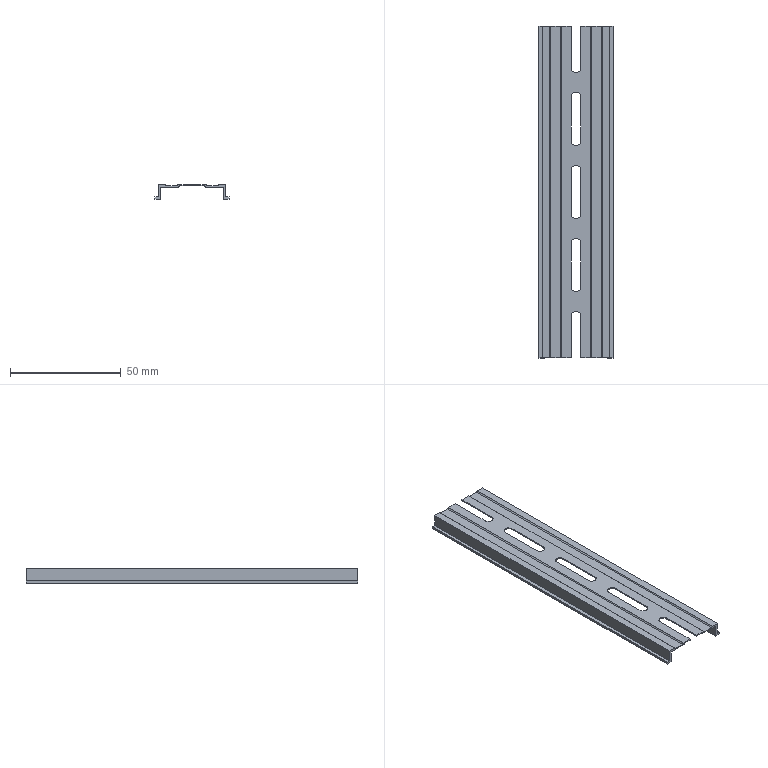Part | STEP file | Mounting plate 1 | 1 solid | 46 faces | box 33.46 x 150 x 6.5 mm | volume 4759 mm3 | plane 32 | cylinder 14 | commonest cylinder face diameters 4.2 x8 1 x6